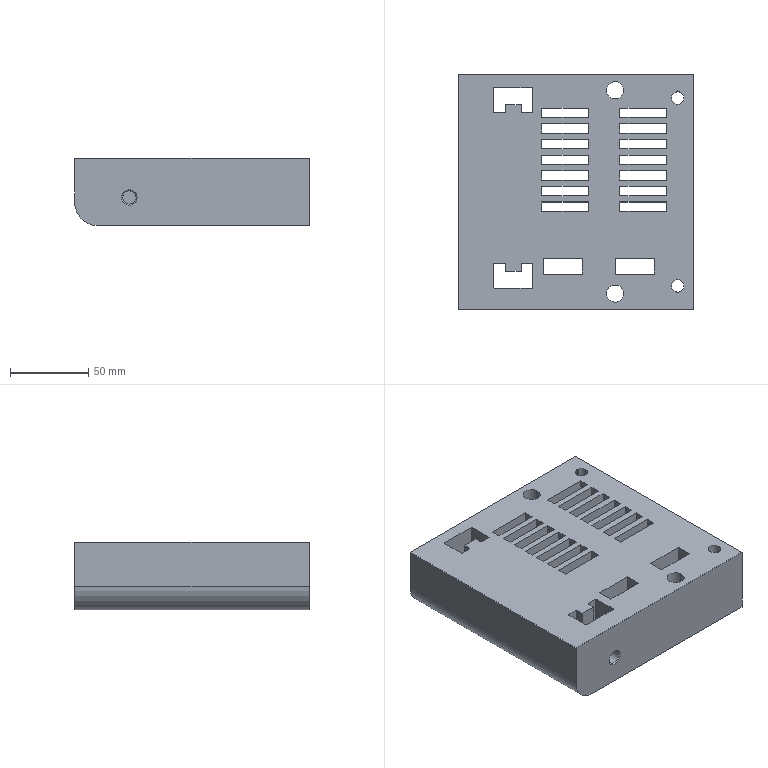Part | STEP file | 1 solid | 118 faces | box 150 x 150 x 43 mm | volume 782567 mm3 | plane 88 | cylinder 27 | cone 3 | commonest cylinder face diameters 1 x18 8.01 x2 8.5 x2 11 x2 17 x2 30 x1